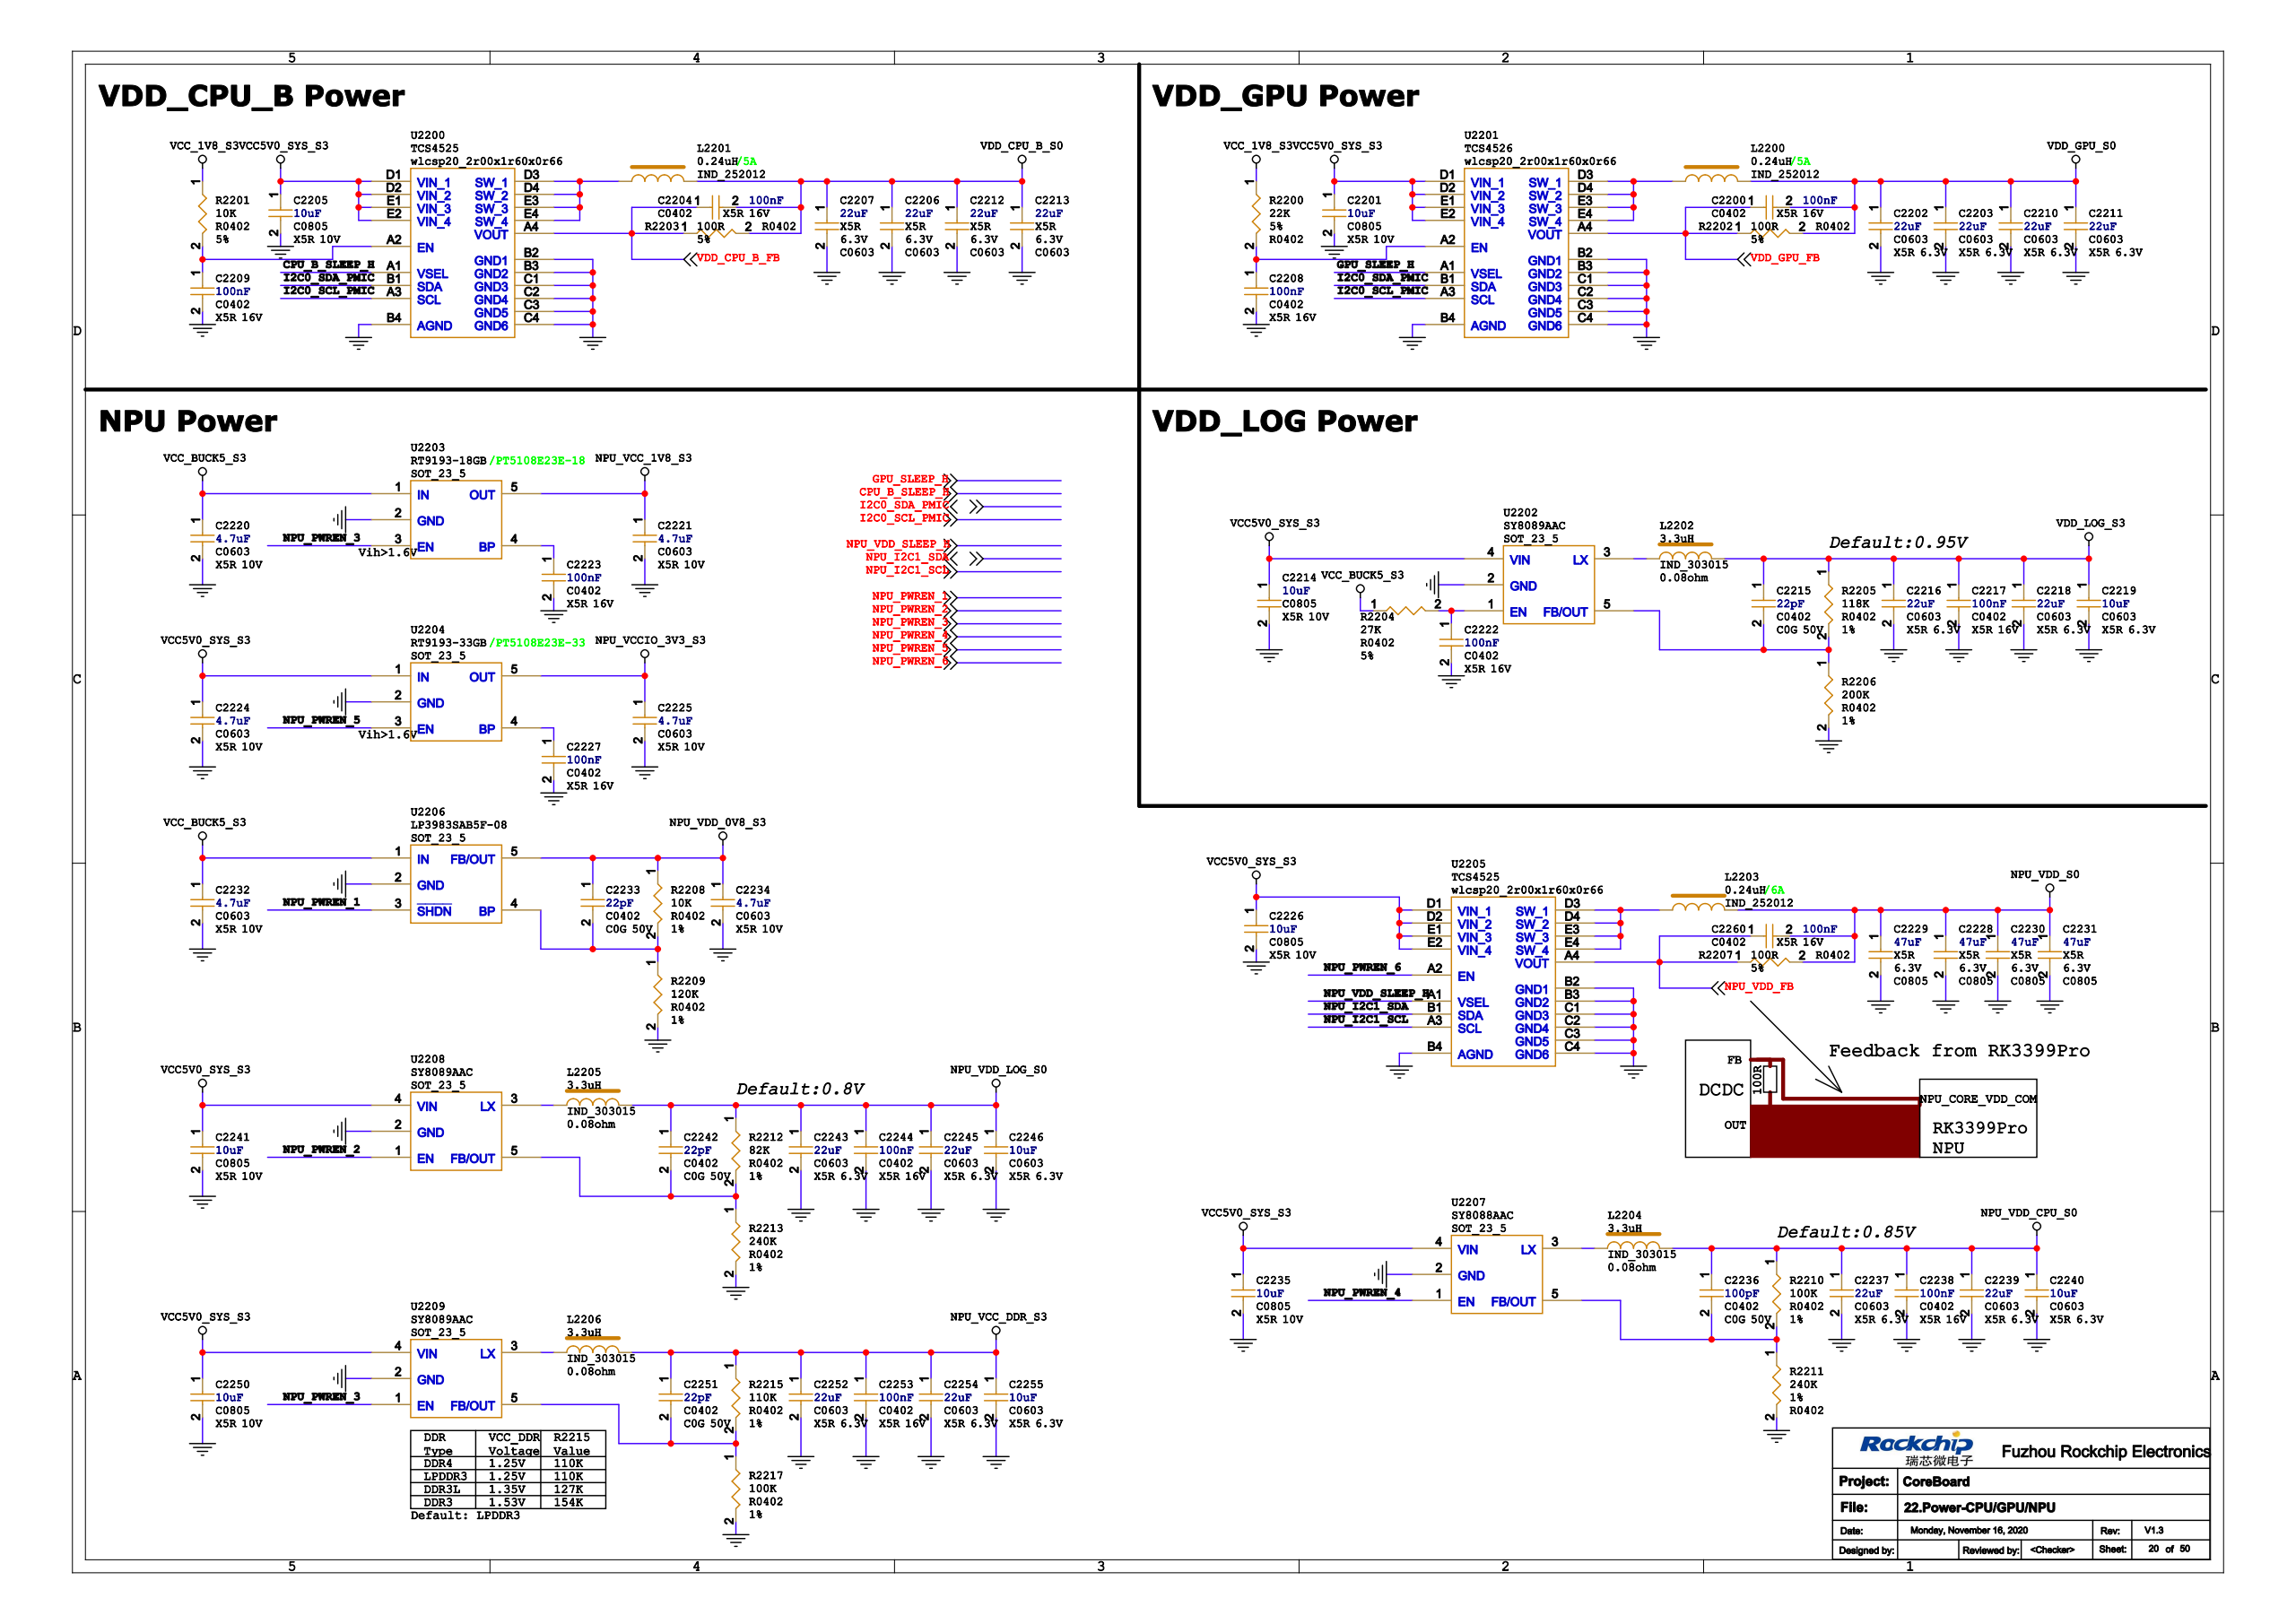Circuit board | Cadence Allegro | 749 parts | 717 nets | one sheet of the schematic
Parts on this sheet (reference | value | footprint):
C2200 | 100nF | C0402
C2201 | 10uF | C0805
C2202 | 22uF | C0603
C2203 | 22uF | C0603
C2204 | 100nF | C0402
C2205 | 10uF | C0805
C2206 | 22uF | C0603
C2207 | 22uF | C0603
C2208 | 100nF | C0402
C2209 | 100nF | C0402
C2210 | 22uF | C0603
C2211 | 22uF | C0603
C2212 | 22uF | C0603
C2213 | 22uF | C0603
C2214 | 10uF | C0805
C2215 | 22pF | C0402
C2216 | 22uF | C0603
C2217 | 100nF | C0402
C2218 | 22uF | C0603
C2219 | 10uF | C0603
C2220 | 4.7uF | C0603
C2221 | 4.7uF | C0603
C2222 | 100nF | C0402
C2223 | 100nF | C0402
C2224 | 4.7uF | C0603
C2225 | 4.7uF | C0603
C2226 | 10uF | C0805
C2227 | 100nF | C0402
C2228 | 47uF | C0805
C2229 | 47uF | C0805
C2230 | 47uF | C0805
C2231 | 47uF | C0805
C2232 | 4.7uF | C0603
C2233 | 22pF | C0402
C2234 | 4.7uF | C0603
C2235 | 10uF | C0805
C2236 | 100pF | C0402
C2237 | 22uF | C0603
C2238 | 100nF | C0402
C2239 | 22uF | C0603
C2240 | 10uF | C0603
C2241 | 10uF | C0805
C2242 | 22pF | C0402
C2243 | 22uF | C0603
C2244 | 100nF | C0402
C2245 | 22uF | C0603
C2246 | 10uF | C0603
C2250 | 10uF | C0805
C2251 | 22pF | C0402
C2252 | 22uF | C0603
C2253 | 100nF | C0402
C2254 | 22uF | C0603
C2255 | 10uF | C0603
C2260 | 100nF | C0402
L2200 | 0.24uH | IND_252012
L2201 | 0.24uH | IND_252012
L2202 | 3.3uH | IND_303015
L2203 | 0.24uH | IND_252012
L2204 | 3.3uH | IND_303015
L2205 | 3.3uH | IND_303015
L2206 | 3.3uH | IND_303015
R2200 | 22K | R0402
R2201 | 10K | R0402
R2202 | 100R | R0402
R2203 | 100R | R0402
R2204 | 27K | R0402
R2205 | 118K | R0402
R2206 | 200K | R0402
R2207 | 100R | R0402
R2208 | 10K | R0402
R2209 | 120K | R0402
R2210 | 100K | R0402
R2211 | 240K | R0402
R2212 | 82K | R0402
R2213 | 240K | R0402
R2215 | 110K | R0402
R2217 | 100K | R0402
U2200 | TCS4525 | WLCSP20_2R00X1R60X0R66
U2201 | TCS4526 | WLCSP20_2R00X1R60X0R66
U2202 | SY8089AAC | SOT_23_5
U2203 | RT9193-18GB | SOT_23_5
U2204 | RT9193-33GB | SOT_23_5
U2205 | TCS4525 | WLCSP20_2R00X1R60X0R66
U2206 | LP3983SAB5F-08 | SOT_23_5
U2207 | SY8088AAC | SOT_23_5
U2208 | SY8089AAC | SOT_23_5
U2209 | SY8089AAC | SOT_23_5
Nets of these parts (net: part-pin ...):
GND: C2201-2 C2202-2 C2203-2 C2205-2 C2206-2 C2207-2 C2208-2 C2209-2 C2210-2 C2211-2 C2212-2 C2213-2 C2214-2 C2216-2 C2217-2 C2218-2 C2219-2 C2220-2 C2221-2 C2222-2 C2223-2 C2224-2 C2225-2 C2226-2 C2227-2 C2228-2 C2229-2 C2230-2 C2231-2 C2232-2 C2234-2 C2235-2 C2237-2 C2238-2 C2239-2 C2240-2 C2241-2 C2243-2 C2244-2 C2245-2 C2246-2 C2250-2 C2252-2 C2253-2 C2254-2 C2255-2 R2206-2 R2209-2 R2211-2 R2213-2 R2217-2 U2200-B2 U2200-B3 U2200-B4 U2200-C1 U2200-C2 U2200-C3 U2200-C4 U2201-B2 U2201-B3 U2201-B4 U2201-C1 U2201-C2 U2201-C3 U2201-C4 U2202-2 U2203-2 U2204-2 U2205-B2 U2205-B3 U2205-B4 U2205-C1 U2205-C2 U2205-C3 U2205-C4 U2206-2 U2207-2 U2208-2 U2209-2
NPU_VCCIO_3V3_S3: C2225-1 U2204-5
VCC5V0_SYS_S3: C2201-1 C2205-1 C2214-1 C2224-1 C2226-1 C2235-1 C2241-1 C2250-1 U2200-D1 U2200-D2 U2200-E1 U2200-E2 U2201-D1 U2201-D2 U2201-E1 U2201-E2 U2202-4 U2204-1 U2205-D1 U2205-D2 U2205-E1 U2205-E2 U2207-4 U2208-4 U2209-4
VDD_LOG_S3: C2215-1 C2216-1 C2217-1 C2218-1 C2219-1 L2202-2 R2205-1
N81509677: C2215-2 R2205-2 R2206-1 U2202-5
NPU_VDD_0V8_S3: C2233-1 C2234-1 R2208-1 U2206-5
N16941445: C2233-2 R2208-2 R2209-1 U2206-4
NPU_VDD_LOG_S0: C2242-1 C2243-1 C2244-1 C2245-1 C2246-1 L2205-2 R2212-1
N81478888: C2242-2 R2212-2 R2213-1 U2208-5
NPU_VCC_DDR_S3: C2251-1 C2252-1 C2253-1 C2254-1 C2255-1 L2206-2 R2215-1
N79991010: C2251-2 R2215-2 R2217-1 U2209-5
NPU_VDD_CPU_S0: C2236-1 C2237-1 C2238-1 C2239-1 C2240-1 L2204-2 R2210-1
N79985256: C2236-2 R2210-2 R2211-1 U2207-5
VCC_BUCK5_S3: C2220-1 C2232-1 R2204-1 U2203-1 U2206-1
NPU_VCC_1V8_S3: C2221-1 U2203-5
NPU_VDD_S0: C2228-1 C2229-1 C2230-1 C2231-1 C2260-2 L2203-2 R2207-2
N78341282: L2200-1 U2201-D3 U2201-D4 U2201-E3 U2201-E4
VDD_GPU_S0: C2200-2 C2202-1 C2203-1 C2210-1 C2211-1 L2200-2 R2202-2
N78340621: L2201-1 U2200-D3 U2200-D4 U2200-E3 U2200-E4
VDD_CPU_B_S0: C2204-2 C2206-1 C2207-1 C2212-1 C2213-1 L2201-2 R2203-2
N81483301: L2203-1 U2205-D3 U2205-D4 U2205-E3 U2205-E4
N81509679: L2202-1 U2202-3
N79985264: L2204-1 U2207-3
N81478894: L2205-1 U2208-3
N79991018: L2206-1 U2209-3
VCC_1V8_S3: R2200-1 R2201-1
N78341328: C2208-1 R2200-2 U2201-A2
N81509890: C2222-1 R2204-2 U2202-1
NPU_PWREN_2: U2208-1
NPU_PWREN_3: U2203-3 U2209-1
NPU_PWREN_1: U2206-3
GPU_SLEEP_H: U2201-A1
CPU_B_SLEEP_H: U2200-A1
I2C0_SDA_PMIC: U2200-B1 U2201-B1
I2C0_SCL_PMIC: U2200-A3 U2201-A3
NPU_PWREN_4: U2207-1
NPU_PWREN_5: U2204-3
NPU_PWREN_6: U2205-A2
VDD_CPU_B_FB: C2204-1 R2203-1 U2200-A4
VDD_GPU_FB: C2200-1 R2202-1 U2201-A4
NPU_I2C1_SCL: U2205-A3
NPU_I2C1_SDA: U2205-B1
NPU_VDD_SLEEP_H: U2205-A1
NPU_VDD_FB: C2260-1 R2207-1 U2205-A4
N78340690: C2209-1 R2201-2 U2200-A2
N81485482: C2223-1 U2203-4
N81485563: C2227-1 U2204-4